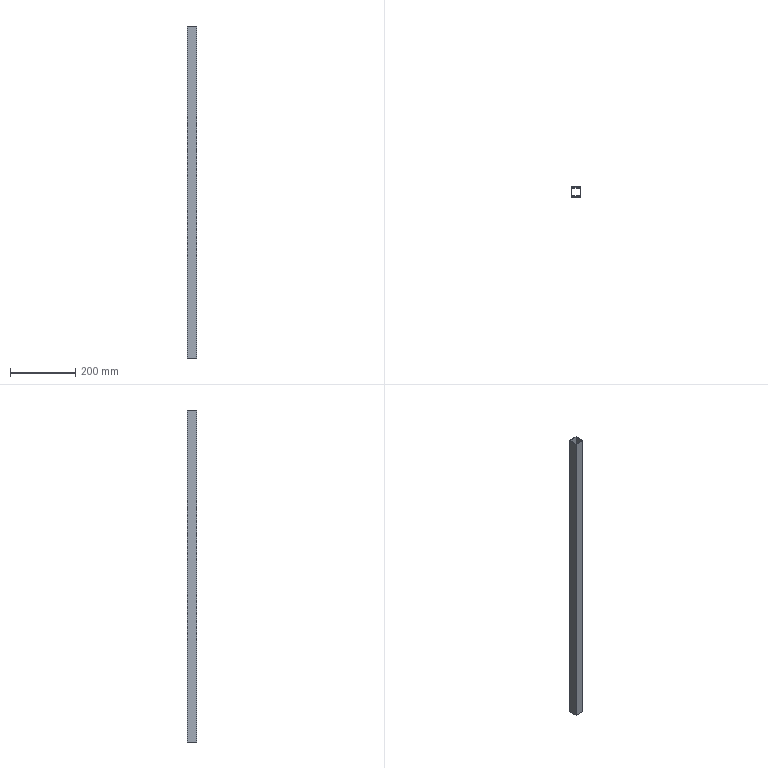Part | SolidWorks | features Extrusion 1 | 1 solid | 10 faces | box 30 x 30 x 1020 mm | volume 228480 mm3 | plane 10
STEP:
#1=CARTESIAN_POINT('',(-15.,15.,510.));
#2=VERTEX_POINT('',#1);
#3=CARTESIAN_POINT('',(-15.,-15.,510.));
#4=VERTEX_POINT('',#3);
#5=CARTESIAN_POINT('',(-15.,-15.,510.));
#6=DIRECTION('',(0.,-1.,0.));
#7=VECTOR('',#6,1000.);
#8=LINE('',#5,#7);
#9=EDGE_CURVE('',#2,#4,#8,.T.);
#10=ORIENTED_EDGE('',*,*,#9,.T.);
#11=CARTESIAN_POINT('',(15.,-15.,510.));
#12=VERTEX_POINT('',#11);
#13=CARTESIAN_POINT('',(15.,-15.,510.));
#14=DIRECTION('',(1.,0.,0.));
#15=VECTOR('',#14,1000.);
#16=LINE('',#13,#15);
#17=EDGE_CURVE('',#4,#12,#16,.T.);
#18=ORIENTED_EDGE('',*,*,#17,.T.);
#19=CARTESIAN_POINT('',(15.,15.,510.));
#20=VERTEX_POINT('',#19);
#21=CARTESIAN_POINT('',(15.,-15.,510.));
#22=DIRECTION('',(0.,1.,0.));
#23=VECTOR('',#22,1000.);
#24=LINE('',#21,#23);
#25=EDGE_CURVE('',#12,#20,#24,.T.);
#26=ORIENTED_EDGE('',*,*,#25,.T.);
#27=CARTESIAN_POINT('',(15.,15.,510.));
#28=DIRECTION('',(-1.,0.,0.));
#29=VECTOR('',#28,1000.);
#30=LINE('',#27,#29);
#31=EDGE_CURVE('',#20,#2,#30,.T.);
#32=ORIENTED_EDGE('',*,*,#31,.T.);
#33=EDGE_LOOP('',(#10,#18,#26,#32));
#34=FACE_OUTER_BOUND('',#33,.T.);
#35=CARTESIAN_POINT('',(13.,13.,510.));
#36=VERTEX_POINT('',#35);
#37=CARTESIAN_POINT('',(-13.,13.,510.));
#38=VERTEX_POINT('',#37);
#39=CARTESIAN_POINT('',(13.,13.,510.));
#40=DIRECTION('',(-1.,0.,0.));
#41=VECTOR('',#40,1000.);
#42=LINE('',#39,#41);
#43=EDGE_CURVE('',#36,#38,#42,.T.);
#44=ORIENTED_EDGE('',*,*,#43,.F.);
#45=CARTESIAN_POINT('',(13.,-13.,510.));
#46=VERTEX_POINT('',#45);
#47=CARTESIAN_POINT('',(13.,-13.,510.));
#48=DIRECTION('',(0.,1.,0.));
#49=VECTOR('',#48,1000.);
#50=LINE('',#47,#49);
#51=EDGE_CURVE('',#46,#36,#50,.T.);
#52=ORIENTED_EDGE('',*,*,#51,.F.);
#53=CARTESIAN_POINT('',(-13.,-13.,510.));
#54=VERTEX_POINT('',#53);
#55=CARTESIAN_POINT('',(13.,-13.,510.));
#56=DIRECTION('',(1.,0.,0.));
#57=VECTOR('',#56,1000.);
#58=LINE('',#55,#57);
#59=EDGE_CURVE('',#54,#46,#58,.T.);
#60=ORIENTED_EDGE('',*,*,#59,.F.);
#61=CARTESIAN_POINT('',(-13.,-13.,510.));
#62=DIRECTION('',(0.,-1.,0.));
#63=VECTOR('',#62,1000.);
#64=LINE('',#61,#63);
#65=EDGE_CURVE('',#38,#54,#64,.T.);
#66=ORIENTED_EDGE('',*,*,#65,.F.);
#67=EDGE_LOOP('',(#44,#52,#60,#66));
#68=FACE_BOUND('',#67,.T.);
#69=CARTESIAN_POINT('',(0.,0.,510.));
#70=DIRECTION('',(0.,0.,1.));
#71=DIRECTION('',(1.,0.,0.));
#72=AXIS2_PLACEMENT_3D('',#69,#70,#71);
#73=PLANE('',#72);
#74=ADVANCED_FACE('',(#34,#68),#73,.T.);
#75=CARTESIAN_POINT('',(-15.,15.,-510.));
#76=VERTEX_POINT('',#75);
#77=CARTESIAN_POINT('',(-15.,-15.,-510.));
#78=VERTEX_POINT('',#77);
#79=CARTESIAN_POINT('',(-15.,-15.,-510.));
#80=DIRECTION('',(0.,-1.,0.));
#81=VECTOR('',#80,1000.);
#82=LINE('',#79,#81);
#83=EDGE_CURVE('',#76,#78,#82,.T.);
#84=ORIENTED_EDGE('',*,*,#83,.F.);
#85=CARTESIAN_POINT('',(15.,15.,-510.));
#86=VERTEX_POINT('',#85);
#87=CARTESIAN_POINT('',(15.,15.,-510.));
#88=DIRECTION('',(-1.,0.,0.));
#89=VECTOR('',#88,1000.);
#90=LINE('',#87,#89);
#91=EDGE_CURVE('',#86,#76,#90,.T.);
#92=ORIENTED_EDGE('',*,*,#91,.F.);
#93=CARTESIAN_POINT('',(15.,-15.,-510.));
#94=VERTEX_POINT('',#93);
#95=CARTESIAN_POINT('',(15.,-15.,-510.));
#96=DIRECTION('',(0.,1.,0.));
#97=VECTOR('',#96,1000.);
#98=LINE('',#95,#97);
#99=EDGE_CURVE('',#94,#86,#98,.T.);
#100=ORIENTED_EDGE('',*,*,#99,.F.);
#101=CARTESIAN_POINT('',(15.,-15.,-510.));
#102=DIRECTION('',(1.,0.,0.));
#103=VECTOR('',#102,1000.);
#104=LINE('',#101,#103);
#105=EDGE_CURVE('',#78,#94,#104,.T.);
#106=ORIENTED_EDGE('',*,*,#105,.F.);
#107=EDGE_LOOP('',(#84,#92,#100,#106));
#108=FACE_OUTER_BOUND('',#107,.T.);
#109=CARTESIAN_POINT('',(13.,-13.,-510.));
#110=VERTEX_POINT('',#109);
#111=CARTESIAN_POINT('',(13.,13.,-510.));
#112=VERTEX_POINT('',#111);
#113=CARTESIAN_POINT('',(13.,-13.,-510.));
#114=DIRECTION('',(0.,1.,0.));
#115=VECTOR('',#114,1000.);
#116=LINE('',#113,#115);
#117=EDGE_CURVE('',#110,#112,#116,.T.);
#118=ORIENTED_EDGE('',*,*,#117,.T.);
#119=CARTESIAN_POINT('',(-13.,13.,-510.));
#120=VERTEX_POINT('',#119);
#121=CARTESIAN_POINT('',(13.,13.,-510.));
#122=DIRECTION('',(-1.,0.,0.));
#123=VECTOR('',#122,1000.);
#124=LINE('',#121,#123);
#125=EDGE_CURVE('',#112,#120,#124,.T.);
#126=ORIENTED_EDGE('',*,*,#125,.T.);
#127=CARTESIAN_POINT('',(-13.,-13.,-510.));
#128=VERTEX_POINT('',#127);
#129=CARTESIAN_POINT('',(-13.,-13.,-510.));
#130=DIRECTION('',(0.,-1.,0.));
#131=VECTOR('',#130,1000.);
#132=LINE('',#129,#131);
#133=EDGE_CURVE('',#120,#128,#132,.T.);
#134=ORIENTED_EDGE('',*,*,#133,.T.);
#135=CARTESIAN_POINT('',(13.,-13.,-510.));
#136=DIRECTION('',(1.,0.,0.));
#137=VECTOR('',#136,1000.);
#138=LINE('',#135,#137);
#139=EDGE_CURVE('',#128,#110,#138,.T.);
#140=ORIENTED_EDGE('',*,*,#139,.T.);
#141=EDGE_LOOP('',(#118,#126,#134,#140));
#142=FACE_BOUND('',#141,.T.);
#143=CARTESIAN_POINT('',(0.,0.,-510.));
#144=DIRECTION('',(0.,0.,1.));
#145=DIRECTION('',(1.,0.,0.));
#146=AXIS2_PLACEMENT_3D('',#143,#144,#145);
#147=PLANE('',#146);
#148=ADVANCED_FACE('',(#108,#142),#147,.F.);
#149=ORIENTED_EDGE('',*,*,#83,.T.);
#150=CARTESIAN_POINT('',(-15.,-15.,510.));
#151=DIRECTION('',(0.,0.,-1.));
#152=VECTOR('',#151,1000.);
#153=LINE('',#150,#152);
#154=EDGE_CURVE('',#4,#78,#153,.T.);
#155=ORIENTED_EDGE('',*,*,#154,.F.);
#156=ORIENTED_EDGE('',*,*,#9,.F.);
#157=CARTESIAN_POINT('',(-15.,15.,510.));
#158=DIRECTION('',(0.,0.,-1.));
#159=VECTOR('',#158,1000.);
#160=LINE('',#157,#159);
#161=EDGE_CURVE('',#2,#76,#160,.T.);
#162=ORIENTED_EDGE('',*,*,#161,.T.);
#163=EDGE_LOOP('',(#149,#155,#156,#162));
#164=FACE_OUTER_BOUND('',#163,.T.);
#165=CARTESIAN_POINT('',(-15.,-15.,510.));
#166=DIRECTION('',(1.,0.,0.));
#167=DIRECTION('',(0.,1.,0.));
#168=AXIS2_PLACEMENT_3D('',#165,#166,#167);
#169=PLANE('',#168);
#170=ADVANCED_FACE('',(#164),#169,.F.);
#171=ORIENTED_EDGE('',*,*,#105,.T.);
#172=CARTESIAN_POINT('',(15.,-15.,510.));
#173=DIRECTION('',(0.,0.,-1.));
#174=VECTOR('',#173,1000.);
#175=LINE('',#172,#174);
#176=EDGE_CURVE('',#12,#94,#175,.T.);
#177=ORIENTED_EDGE('',*,*,#176,.F.);
#178=ORIENTED_EDGE('',*,*,#17,.F.);
#179=ORIENTED_EDGE('',*,*,#154,.T.);
#180=EDGE_LOOP('',(#171,#177,#178,#179));
#181=FACE_OUTER_BOUND('',#180,.T.);
#182=CARTESIAN_POINT('',(15.,-15.,510.));
#183=DIRECTION('',(0.,1.,0.));
#184=DIRECTION('',(-1.,0.,0.));
#185=AXIS2_PLACEMENT_3D('',#182,#183,#184);
#186=PLANE('',#185);
#187=ADVANCED_FACE('',(#181),#186,.F.);
#188=ORIENTED_EDGE('',*,*,#99,.T.);
#189=CARTESIAN_POINT('',(15.,15.,510.));
#190=DIRECTION('',(0.,0.,-1.));
#191=VECTOR('',#190,1000.);
#192=LINE('',#189,#191);
#193=EDGE_CURVE('',#20,#86,#192,.T.);
#194=ORIENTED_EDGE('',*,*,#193,.F.);
#195=ORIENTED_EDGE('',*,*,#25,.F.);
#196=ORIENTED_EDGE('',*,*,#176,.T.);
#197=EDGE_LOOP('',(#188,#194,#195,#196));
#198=FACE_OUTER_BOUND('',#197,.T.);
#199=CARTESIAN_POINT('',(15.,-15.,510.));
#200=DIRECTION('',(-1.,0.,0.));
#201=DIRECTION('',(0.,0.,1.));
#202=AXIS2_PLACEMENT_3D('',#199,#200,#201);
#203=PLANE('',#202);
#204=ADVANCED_FACE('',(#198),#203,.F.);
#205=ORIENTED_EDGE('',*,*,#91,.T.);
#206=ORIENTED_EDGE('',*,*,#161,.F.);
#207=ORIENTED_EDGE('',*,*,#31,.F.);
#208=ORIENTED_EDGE('',*,*,#193,.T.);
#209=EDGE_LOOP('',(#205,#206,#207,#208));
#210=FACE_OUTER_BOUND('',#209,.T.);
#211=CARTESIAN_POINT('',(15.,15.,510.));
#212=DIRECTION('',(0.,-1.,0.));
#213=DIRECTION('',(0.,0.,-1.));
#214=AXIS2_PLACEMENT_3D('',#211,#212,#213);
#215=PLANE('',#214);
#216=ADVANCED_FACE('',(#210),#215,.F.);
#217=ORIENTED_EDGE('',*,*,#117,.F.);
#218=CARTESIAN_POINT('',(13.,-13.,510.));
#219=DIRECTION('',(0.,0.,-1.));
#220=VECTOR('',#219,1000.);
#221=LINE('',#218,#220);
#222=EDGE_CURVE('',#46,#110,#221,.T.);
#223=ORIENTED_EDGE('',*,*,#222,.F.);
#224=ORIENTED_EDGE('',*,*,#51,.T.);
#225=CARTESIAN_POINT('',(13.,13.,510.));
#226=DIRECTION('',(0.,0.,-1.));
#227=VECTOR('',#226,1000.);
#228=LINE('',#225,#227);
#229=EDGE_CURVE('',#36,#112,#228,.T.);
#230=ORIENTED_EDGE('',*,*,#229,.T.);
#231=EDGE_LOOP('',(#217,#223,#224,#230));
#232=FACE_OUTER_BOUND('',#231,.T.);
#233=CARTESIAN_POINT('',(13.,-13.,510.));
#234=DIRECTION('',(-1.,0.,0.));
#235=DIRECTION('',(0.,0.,1.));
#236=AXIS2_PLACEMENT_3D('',#233,#234,#235);
#237=PLANE('',#236);
#238=ADVANCED_FACE('',(#232),#237,.T.);
#239=ORIENTED_EDGE('',*,*,#125,.F.);
#240=ORIENTED_EDGE('',*,*,#229,.F.);
#241=ORIENTED_EDGE('',*,*,#43,.T.);
#242=CARTESIAN_POINT('',(-13.,13.,510.));
#243=DIRECTION('',(0.,0.,-1.));
#244=VECTOR('',#243,1000.);
#245=LINE('',#242,#244);
#246=EDGE_CURVE('',#38,#120,#245,.T.);
#247=ORIENTED_EDGE('',*,*,#246,.T.);
#248=EDGE_LOOP('',(#239,#240,#241,#247));
#249=FACE_OUTER_BOUND('',#248,.T.);
#250=CARTESIAN_POINT('',(13.,13.,510.));
#251=DIRECTION('',(0.,-1.,0.));
#252=DIRECTION('',(1.,0.,0.));
#253=AXIS2_PLACEMENT_3D('',#250,#251,#252);
#254=PLANE('',#253);
#255=ADVANCED_FACE('',(#249),#254,.T.);
#256=ORIENTED_EDGE('',*,*,#133,.F.);
#257=ORIENTED_EDGE('',*,*,#246,.F.);
#258=ORIENTED_EDGE('',*,*,#65,.T.);
#259=CARTESIAN_POINT('',(-13.,-13.,510.));
#260=DIRECTION('',(0.,0.,-1.));
#261=VECTOR('',#260,1000.);
#262=LINE('',#259,#261);
#263=EDGE_CURVE('',#54,#128,#262,.T.);
#264=ORIENTED_EDGE('',*,*,#263,.T.);
#265=EDGE_LOOP('',(#256,#257,#258,#264));
#266=FACE_OUTER_BOUND('',#265,.T.);
#267=CARTESIAN_POINT('',(-13.,-13.,510.));
#268=DIRECTION('',(1.,0.,0.));
#269=DIRECTION('',(0.,1.,0.));
#270=AXIS2_PLACEMENT_3D('',#267,#268,#269);
#271=PLANE('',#270);
#272=ADVANCED_FACE('',(#266),#271,.T.);
#273=ORIENTED_EDGE('',*,*,#139,.F.);
#274=ORIENTED_EDGE('',*,*,#263,.F.);
#275=ORIENTED_EDGE('',*,*,#59,.T.);
#276=ORIENTED_EDGE('',*,*,#222,.T.);
#277=EDGE_LOOP('',(#273,#274,#275,#276));
#278=FACE_OUTER_BOUND('',#277,.T.);
#279=CARTESIAN_POINT('',(13.,-13.,510.));
#280=DIRECTION('',(0.,1.,0.));
#281=DIRECTION('',(-1.,0.,0.));
#282=AXIS2_PLACEMENT_3D('',#279,#280,#281);
#283=PLANE('',#282);
#284=ADVANCED_FACE('',(#278),#283,.T.);
#285=CLOSED_SHELL('',(#74,#148,#170,#187,#204,#216,#238,#255,#272,#284));
#286=MANIFOLD_SOLID_BREP('',#285);
#287=CARTESIAN_POINT('',(0.,0.,0.));
#288=DIRECTION('',(0.,0.,1.));
#289=DIRECTION('',(1.,0.,0.));
#290=AXIS2_PLACEMENT_3D('',#287,#288,#289);
#291=(LENGTH_UNIT()NAMED_UNIT(*)SI_UNIT(.MILLI.,.METRE.));
#292=UNCERTAINTY_MEASURE_WITH_UNIT(LENGTH_MEASURE(0.00001),#291,'','');
#293=(NAMED_UNIT(*)PLANE_ANGLE_UNIT()SI_UNIT($,.RADIAN.));
#294=(NAMED_UNIT(*)SI_UNIT($,.STERADIAN.)SOLID_ANGLE_UNIT());
#295=(GEOMETRIC_REPRESENTATION_CONTEXT(3)GLOBAL_UNCERTAINTY_ASSIGNED_CONTEXT((#292))GLOBAL_UNIT_ASSIGNED_CONTEXT((#291,#293,#294))REPRESENTATION_CONTEXT('',''));
#296=ADVANCED_BREP_SHAPE_REPRESENTATION('',(#286,#290),#295);